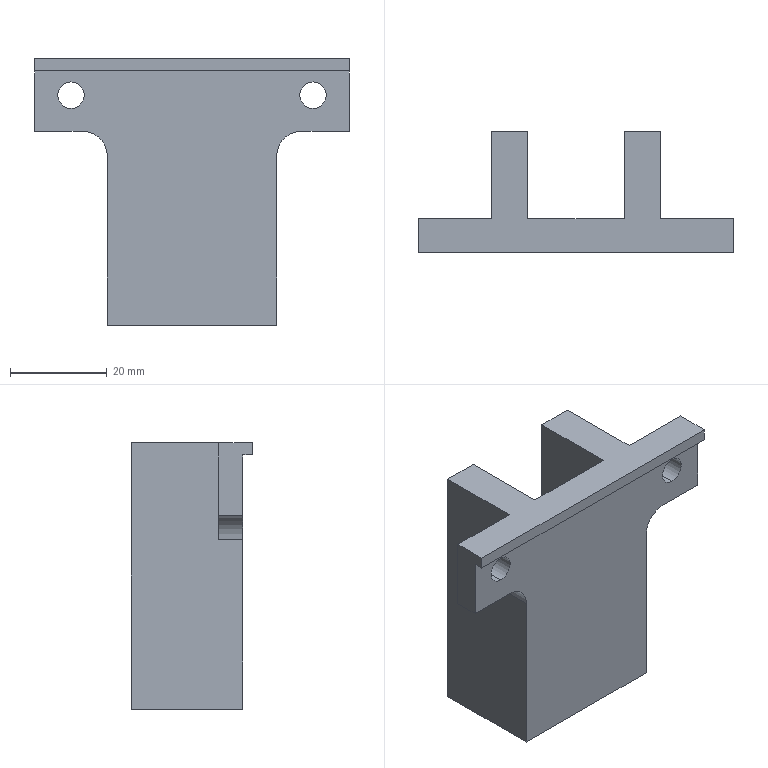Part | STEP file | Sliding fork | 1 solid | 24 faces | box 65 x 25 x 55 mm | volume 26866 mm3 | plane 18 | cylinder 6 | commonest cylinder face diameters 5.5 x4 10 x2